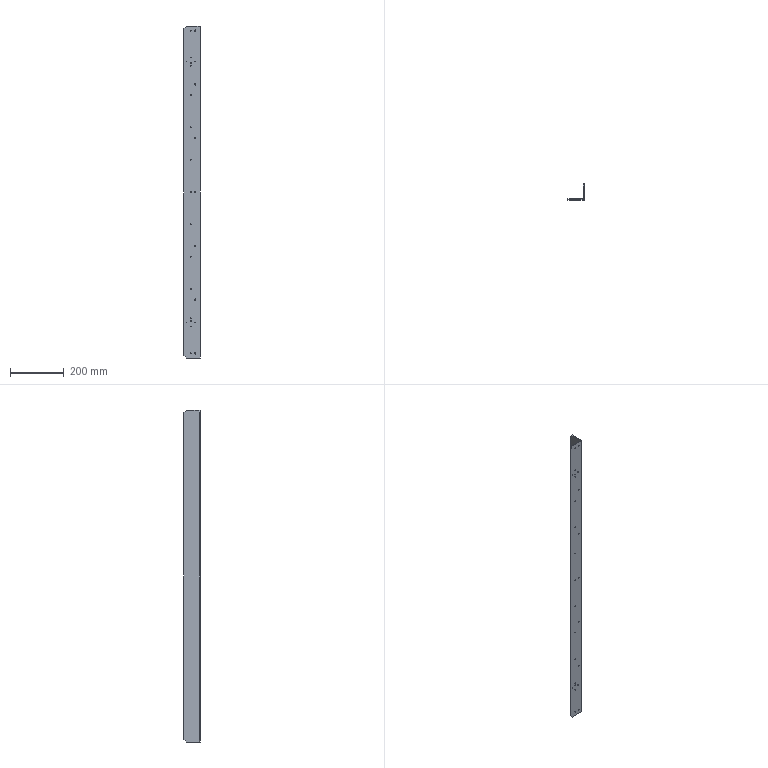Part | SolidWorks | features HoleWzd 4, Chamfer 1, Extrusion 1 | 1 solid | 64 faces | box 60 x 60 x 1234 mm | volume 431666 mm3 | cylinder 52 | plane 12 | commonest cylinder face diameters 3.3 x38 4.8 x14